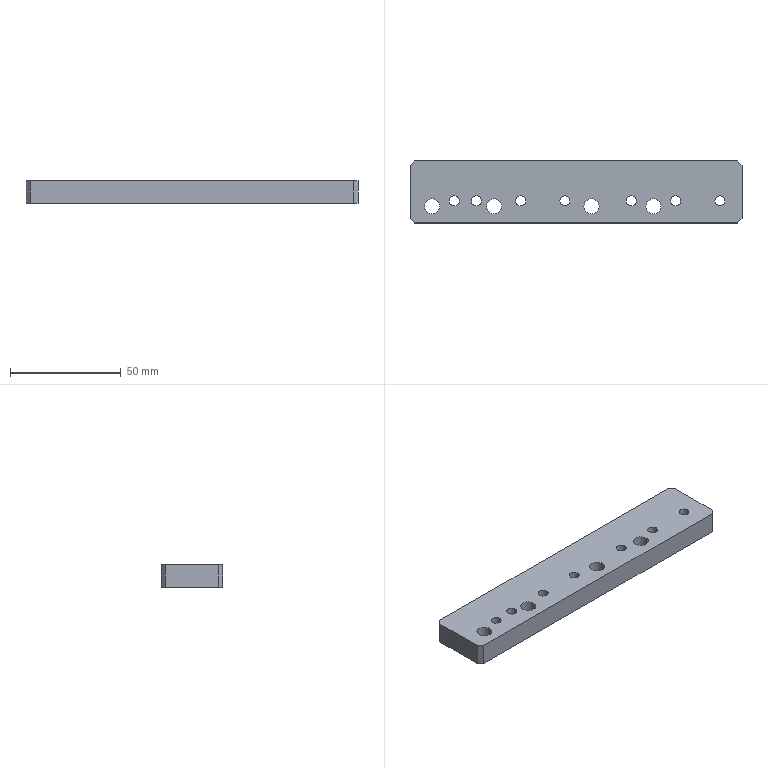Part | STEP file | PN_0010 | 1 solid | 53 faces | box 150 x 28 x 10 mm | volume 38296 mm3 | cylinder 36 | plane 17 | commonest cylinder face diameters 4.5 x14 8 x14 6.8 x8